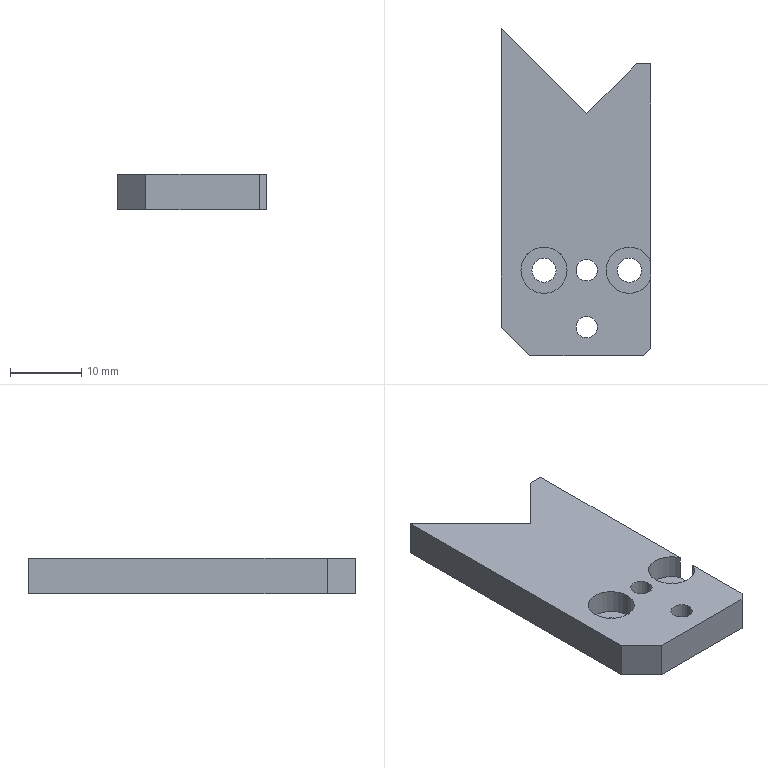Part | STEP file | 11-FG-E02611 | 1 solid | 23 faces | box 21 x 46 x 5 mm | volume 3756 mm3 | plane 12 | cylinder 11 | commonest cylinder face diameters 3 x4 3.4 x4 6.5 x3
STEP:
#1=CARTESIAN_POINT('',(1.5,-9.5,0.));
#2=VERTEX_POINT('',#1);
#3=CARTESIAN_POINT('',(-1.5,-9.5,0.));
#4=VERTEX_POINT('',#3);
#5=CARTESIAN_POINT('',(0.,-9.5,0.));
#6=DIRECTION('',(0.,0.,-1.));
#7=DIRECTION('',(-1.,0.,0.));
#8=AXIS2_PLACEMENT_3D('',#5,#6,#7);
#9=CIRCLE('',#8,1.5);
#10=EDGE_CURVE('',#2,#4,#9,.T.);
#11=ORIENTED_EDGE('',*,*,#10,.T.);
#12=CARTESIAN_POINT('',(-1.5,-9.5,5.));
#13=VERTEX_POINT('',#12);
#14=CARTESIAN_POINT('',(-1.5,-9.5,5.));
#15=DIRECTION('',(0.,0.,1.));
#16=VECTOR('',#15,1000.);
#17=LINE('',#14,#16);
#18=EDGE_CURVE('',#4,#13,#17,.T.);
#19=ORIENTED_EDGE('',*,*,#18,.T.);
#20=CARTESIAN_POINT('',(1.5,-9.5,5.));
#21=VERTEX_POINT('',#20);
#22=CARTESIAN_POINT('',(0.,-9.5,5.));
#23=DIRECTION('',(0.,0.,1.));
#24=DIRECTION('',(1.,0.,0.));
#25=AXIS2_PLACEMENT_3D('',#22,#23,#24);
#26=CIRCLE('',#25,1.5);
#27=EDGE_CURVE('',#13,#21,#26,.T.);
#28=ORIENTED_EDGE('',*,*,#27,.T.);
#29=CARTESIAN_POINT('',(1.5,-9.5,5.));
#30=DIRECTION('',(0.,0.,1.));
#31=VECTOR('',#30,1000.);
#32=LINE('',#29,#31);
#33=EDGE_CURVE('',#2,#21,#32,.T.);
#34=ORIENTED_EDGE('',*,*,#33,.F.);
#35=EDGE_LOOP('',(#11,#19,#28,#34));
#36=FACE_OUTER_BOUND('',#35,.T.);
#37=CARTESIAN_POINT('',(0.,-9.5,5.));
#38=DIRECTION('',(0.,0.,1.));
#39=DIRECTION('',(1.,0.,0.));
#40=AXIS2_PLACEMENT_3D('',#37,#38,#39);
#41=CYLINDRICAL_SURFACE('',#40,1.5);
#42=ADVANCED_FACE('',(#36),#41,.F.);
#43=CARTESIAN_POINT('',(1.5,-17.5,0.));
#44=VERTEX_POINT('',#43);
#45=CARTESIAN_POINT('',(-1.5,-17.5,0.));
#46=VERTEX_POINT('',#45);
#47=CARTESIAN_POINT('',(0.,-17.5,0.));
#48=DIRECTION('',(0.,0.,-1.));
#49=DIRECTION('',(-1.,0.,0.));
#50=AXIS2_PLACEMENT_3D('',#47,#48,#49);
#51=CIRCLE('',#50,1.5);
#52=EDGE_CURVE('',#44,#46,#51,.T.);
#53=ORIENTED_EDGE('',*,*,#52,.T.);
#54=CARTESIAN_POINT('',(-1.5,-17.5,5.));
#55=VERTEX_POINT('',#54);
#56=CARTESIAN_POINT('',(-1.5,-17.5,5.));
#57=DIRECTION('',(0.,0.,1.));
#58=VECTOR('',#57,1000.);
#59=LINE('',#56,#58);
#60=EDGE_CURVE('',#46,#55,#59,.T.);
#61=ORIENTED_EDGE('',*,*,#60,.T.);
#62=CARTESIAN_POINT('',(1.5,-17.5,5.));
#63=VERTEX_POINT('',#62);
#64=CARTESIAN_POINT('',(0.,-17.5,5.));
#65=DIRECTION('',(0.,0.,1.));
#66=DIRECTION('',(1.,0.,0.));
#67=AXIS2_PLACEMENT_3D('',#64,#65,#66);
#68=CIRCLE('',#67,1.5);
#69=EDGE_CURVE('',#55,#63,#68,.T.);
#70=ORIENTED_EDGE('',*,*,#69,.T.);
#71=CARTESIAN_POINT('',(1.5,-17.5,5.));
#72=DIRECTION('',(0.,0.,1.));
#73=VECTOR('',#72,1000.);
#74=LINE('',#71,#73);
#75=EDGE_CURVE('',#44,#63,#74,.T.);
#76=ORIENTED_EDGE('',*,*,#75,.F.);
#77=EDGE_LOOP('',(#53,#61,#70,#76));
#78=FACE_OUTER_BOUND('',#77,.T.);
#79=CARTESIAN_POINT('',(0.,-17.5,5.));
#80=DIRECTION('',(0.,0.,1.));
#81=DIRECTION('',(1.,0.,0.));
#82=AXIS2_PLACEMENT_3D('',#79,#80,#81);
#83=CYLINDRICAL_SURFACE('',#82,1.5);
#84=ADVANCED_FACE('',(#78),#83,.F.);
#85=CARTESIAN_POINT('',(4.3,-9.5,0.));
#86=VERTEX_POINT('',#85);
#87=CARTESIAN_POINT('',(7.7,-9.5,0.));
#88=VERTEX_POINT('',#87);
#89=CARTESIAN_POINT('',(6.,-9.5,0.));
#90=DIRECTION('',(0.,0.,1.));
#91=DIRECTION('',(1.,0.,0.));
#92=AXIS2_PLACEMENT_3D('',#89,#90,#91);
#93=CIRCLE('',#92,1.7);
#94=EDGE_CURVE('',#86,#88,#93,.T.);
#95=ORIENTED_EDGE('',*,*,#94,.F.);
#96=CARTESIAN_POINT('',(4.3,-9.5,1.6));
#97=VERTEX_POINT('',#96);
#98=CARTESIAN_POINT('',(4.3,-9.5,5.));
#99=DIRECTION('',(0.,0.,1.));
#100=VECTOR('',#99,1000.);
#101=LINE('',#98,#100);
#102=EDGE_CURVE('',#86,#97,#101,.T.);
#103=ORIENTED_EDGE('',*,*,#102,.T.);
#104=CARTESIAN_POINT('',(7.7,-9.5,1.6));
#105=VERTEX_POINT('',#104);
#106=CARTESIAN_POINT('',(6.,-9.5,1.6));
#107=DIRECTION('',(0.,0.,1.));
#108=DIRECTION('',(1.,0.,0.));
#109=AXIS2_PLACEMENT_3D('',#106,#107,#108);
#110=CIRCLE('',#109,1.7);
#111=EDGE_CURVE('',#97,#105,#110,.T.);
#112=ORIENTED_EDGE('',*,*,#111,.T.);
#113=CARTESIAN_POINT('',(7.7,-9.5,5.));
#114=DIRECTION('',(0.,0.,1.));
#115=VECTOR('',#114,1000.);
#116=LINE('',#113,#115);
#117=EDGE_CURVE('',#88,#105,#116,.T.);
#118=ORIENTED_EDGE('',*,*,#117,.F.);
#119=EDGE_LOOP('',(#95,#103,#112,#118));
#120=FACE_OUTER_BOUND('',#119,.T.);
#121=CARTESIAN_POINT('',(6.,-9.5,5.));
#122=DIRECTION('',(0.,0.,1.));
#123=DIRECTION('',(1.,0.,0.));
#124=AXIS2_PLACEMENT_3D('',#121,#122,#123);
#125=CYLINDRICAL_SURFACE('',#124,1.7);
#126=ADVANCED_FACE('',(#120),#125,.F.);
#127=CARTESIAN_POINT('',(-7.7,-9.5,0.));
#128=VERTEX_POINT('',#127);
#129=CARTESIAN_POINT('',(-4.3,-9.5,0.));
#130=VERTEX_POINT('',#129);
#131=CARTESIAN_POINT('',(-6.,-9.5,0.));
#132=DIRECTION('',(0.,0.,1.));
#133=DIRECTION('',(1.,0.,0.));
#134=AXIS2_PLACEMENT_3D('',#131,#132,#133);
#135=CIRCLE('',#134,1.7);
#136=EDGE_CURVE('',#128,#130,#135,.T.);
#137=ORIENTED_EDGE('',*,*,#136,.F.);
#138=CARTESIAN_POINT('',(-7.7,-9.5,1.6));
#139=VERTEX_POINT('',#138);
#140=CARTESIAN_POINT('',(-7.7,-9.5,5.));
#141=DIRECTION('',(0.,0.,1.));
#142=VECTOR('',#141,1000.);
#143=LINE('',#140,#142);
#144=EDGE_CURVE('',#128,#139,#143,.T.);
#145=ORIENTED_EDGE('',*,*,#144,.T.);
#146=CARTESIAN_POINT('',(-4.3,-9.5,1.6));
#147=VERTEX_POINT('',#146);
#148=CARTESIAN_POINT('',(-6.,-9.5,1.6));
#149=DIRECTION('',(0.,0.,1.));
#150=DIRECTION('',(1.,0.,0.));
#151=AXIS2_PLACEMENT_3D('',#148,#149,#150);
#152=CIRCLE('',#151,1.7);
#153=EDGE_CURVE('',#139,#147,#152,.T.);
#154=ORIENTED_EDGE('',*,*,#153,.T.);
#155=CARTESIAN_POINT('',(-4.3,-9.5,5.));
#156=DIRECTION('',(0.,0.,1.));
#157=VECTOR('',#156,1000.);
#158=LINE('',#155,#157);
#159=EDGE_CURVE('',#130,#147,#158,.T.);
#160=ORIENTED_EDGE('',*,*,#159,.F.);
#161=EDGE_LOOP('',(#137,#145,#154,#160));
#162=FACE_OUTER_BOUND('',#161,.T.);
#163=CARTESIAN_POINT('',(-6.,-9.5,5.));
#164=DIRECTION('',(0.,0.,1.));
#165=DIRECTION('',(1.,0.,0.));
#166=AXIS2_PLACEMENT_3D('',#163,#164,#165);
#167=CYLINDRICAL_SURFACE('',#166,1.7);
#168=ADVANCED_FACE('',(#162),#167,.F.);
#169=CARTESIAN_POINT('',(-9.25,-9.5,1.6));
#170=VERTEX_POINT('',#169);
#171=CARTESIAN_POINT('',(-2.75,-9.5,1.6));
#172=VERTEX_POINT('',#171);
#173=CARTESIAN_POINT('',(-6.,-9.5,1.6));
#174=DIRECTION('',(0.,0.,1.));
#175=DIRECTION('',(1.,0.,0.));
#176=AXIS2_PLACEMENT_3D('',#173,#174,#175);
#177=CIRCLE('',#176,3.25);
#178=EDGE_CURVE('',#170,#172,#177,.T.);
#179=ORIENTED_EDGE('',*,*,#178,.F.);
#180=CARTESIAN_POINT('',(-9.25,-9.5,5.));
#181=VERTEX_POINT('',#180);
#182=CARTESIAN_POINT('',(-9.25,-9.5,5.));
#183=DIRECTION('',(0.,0.,1.));
#184=VECTOR('',#183,1000.);
#185=LINE('',#182,#184);
#186=EDGE_CURVE('',#170,#181,#185,.T.);
#187=ORIENTED_EDGE('',*,*,#186,.T.);
#188=CARTESIAN_POINT('',(-2.75,-9.5,5.));
#189=VERTEX_POINT('',#188);
#190=CARTESIAN_POINT('',(-6.,-9.5,5.));
#191=DIRECTION('',(0.,0.,1.));
#192=DIRECTION('',(1.,0.,0.));
#193=AXIS2_PLACEMENT_3D('',#190,#191,#192);
#194=CIRCLE('',#193,3.25);
#195=EDGE_CURVE('',#181,#189,#194,.T.);
#196=ORIENTED_EDGE('',*,*,#195,.T.);
#197=CARTESIAN_POINT('',(-2.75,-9.5,5.));
#198=DIRECTION('',(0.,0.,1.));
#199=VECTOR('',#198,1000.);
#200=LINE('',#197,#199);
#201=EDGE_CURVE('',#172,#189,#200,.T.);
#202=ORIENTED_EDGE('',*,*,#201,.F.);
#203=EDGE_LOOP('',(#179,#187,#196,#202));
#204=FACE_OUTER_BOUND('',#203,.T.);
#205=CARTESIAN_POINT('',(-6.,-9.5,5.));
#206=DIRECTION('',(0.,0.,1.));
#207=DIRECTION('',(1.,0.,0.));
#208=AXIS2_PLACEMENT_3D('',#205,#206,#207);
#209=CYLINDRICAL_SURFACE('',#208,3.25);
#210=ADVANCED_FACE('',(#204),#209,.F.);
#211=CARTESIAN_POINT('',(-6.,-9.5,5.));
#212=DIRECTION('',(0.,0.,1.));
#213=DIRECTION('',(1.,0.,0.));
#214=AXIS2_PLACEMENT_3D('',#211,#212,#213);
#215=CIRCLE('',#214,3.25);
#216=EDGE_CURVE('',#189,#181,#215,.T.);
#217=ORIENTED_EDGE('',*,*,#216,.F.);
#218=ORIENTED_EDGE('',*,*,#195,.F.);
#219=EDGE_LOOP('',(#217,#218));
#220=FACE_BOUND('',#219,.T.);
#221=CARTESIAN_POINT('',(0.,-9.5,5.));
#222=DIRECTION('',(0.,0.,1.));
#223=DIRECTION('',(1.,0.,0.));
#224=AXIS2_PLACEMENT_3D('',#221,#222,#223);
#225=CIRCLE('',#224,1.5);
#226=EDGE_CURVE('',#21,#13,#225,.T.);
#227=ORIENTED_EDGE('',*,*,#226,.F.);
#228=ORIENTED_EDGE('',*,*,#27,.F.);
#229=EDGE_LOOP('',(#227,#228));
#230=FACE_BOUND('',#229,.T.);
#231=CARTESIAN_POINT('',(0.,-17.5,5.));
#232=DIRECTION('',(0.,0.,1.));
#233=DIRECTION('',(1.,0.,0.));
#234=AXIS2_PLACEMENT_3D('',#231,#232,#233);
#235=CIRCLE('',#234,1.5);
#236=EDGE_CURVE('',#63,#55,#235,.T.);
#237=ORIENTED_EDGE('',*,*,#236,.F.);
#238=ORIENTED_EDGE('',*,*,#69,.F.);
#239=EDGE_LOOP('',(#237,#238));
#240=FACE_BOUND('',#239,.T.);
#241=CARTESIAN_POINT('',(-8.,-21.5,5.));
#242=VERTEX_POINT('',#241);
#243=CARTESIAN_POINT('',(8.,-21.5,5.));
#244=VERTEX_POINT('',#243);
#245=CARTESIAN_POINT('',(-9.,-21.5,5.));
#246=DIRECTION('',(1.,0.,0.));
#247=VECTOR('',#246,1000.);
#248=LINE('',#245,#247);
#249=EDGE_CURVE('',#242,#244,#248,.T.);
#250=ORIENTED_EDGE('',*,*,#249,.T.);
#251=CARTESIAN_POINT('',(9.,-20.5,5.));
#252=VERTEX_POINT('',#251);
#253=CARTESIAN_POINT('',(9.,-20.5,5.));
#254=DIRECTION('',(0.7071,0.7071,0.));
#255=VECTOR('',#254,1000.);
#256=LINE('',#253,#255);
#257=EDGE_CURVE('',#244,#252,#256,.T.);
#258=ORIENTED_EDGE('',*,*,#257,.T.);
#259=CARTESIAN_POINT('',(9.,-10.75,5.));
#260=VERTEX_POINT('',#259);
#261=CARTESIAN_POINT('',(9.,-21.5,5.));
#262=DIRECTION('',(0.,1.,0.));
#263=VECTOR('',#262,1000.);
#264=LINE('',#261,#263);
#265=EDGE_CURVE('',#252,#260,#264,.T.);
#266=ORIENTED_EDGE('',*,*,#265,.T.);
#267=CARTESIAN_POINT('',(9.,-8.25,5.));
#268=VERTEX_POINT('',#267);
#269=CARTESIAN_POINT('',(6.,-9.5,5.));
#270=DIRECTION('',(0.,0.,1.));
#271=DIRECTION('',(1.,0.,0.));
#272=AXIS2_PLACEMENT_3D('',#269,#270,#271);
#273=CIRCLE('',#272,3.25);
#274=EDGE_CURVE('',#268,#260,#273,.T.);
#275=ORIENTED_EDGE('',*,*,#274,.F.);
#276=CARTESIAN_POINT('',(9.,19.5,5.));
#277=VERTEX_POINT('',#276);
#278=CARTESIAN_POINT('',(9.,-21.5,5.));
#279=DIRECTION('',(0.,1.,0.));
#280=VECTOR('',#279,1000.);
#281=LINE('',#278,#280);
#282=EDGE_CURVE('',#268,#277,#281,.T.);
#283=ORIENTED_EDGE('',*,*,#282,.T.);
#284=CARTESIAN_POINT('',(7.,19.5,5.));
#285=VERTEX_POINT('',#284);
#286=CARTESIAN_POINT('',(0.,19.5,5.));
#287=DIRECTION('',(1.,0.,0.));
#288=VECTOR('',#287,1000.);
#289=LINE('',#286,#288);
#290=EDGE_CURVE('',#285,#277,#289,.T.);
#291=ORIENTED_EDGE('',*,*,#290,.F.);
#292=CARTESIAN_POINT('',(0.,12.5,5.));
#293=VERTEX_POINT('',#292);
#294=CARTESIAN_POINT('',(0.,12.5,5.));
#295=DIRECTION('',(0.7071,0.7071,0.));
#296=VECTOR('',#295,1000.);
#297=LINE('',#294,#296);
#298=EDGE_CURVE('',#293,#285,#297,.T.);
#299=ORIENTED_EDGE('',*,*,#298,.F.);
#300=CARTESIAN_POINT('',(-12.,24.5,5.));
#301=VERTEX_POINT('',#300);
#302=CARTESIAN_POINT('',(-9.,21.5,5.));
#303=DIRECTION('',(0.7071,-0.7071,0.));
#304=VECTOR('',#303,1000.);
#305=LINE('',#302,#304);
#306=EDGE_CURVE('',#301,#293,#305,.T.);
#307=ORIENTED_EDGE('',*,*,#306,.F.);
#308=CARTESIAN_POINT('',(-12.,-17.5,5.));
#309=VERTEX_POINT('',#308);
#310=CARTESIAN_POINT('',(-12.,0.,5.));
#311=DIRECTION('',(0.,-1.,0.));
#312=VECTOR('',#311,1000.);
#313=LINE('',#310,#312);
#314=EDGE_CURVE('',#301,#309,#313,.T.);
#315=ORIENTED_EDGE('',*,*,#314,.T.);
#316=CARTESIAN_POINT('',(-8.,-21.5,5.));
#317=DIRECTION('',(0.7071,-0.7071,0.));
#318=VECTOR('',#317,1000.);
#319=LINE('',#316,#318);
#320=EDGE_CURVE('',#309,#242,#319,.T.);
#321=ORIENTED_EDGE('',*,*,#320,.T.);
#322=EDGE_LOOP('',(#250,#258,#266,#275,#283,#291,#299,#307,#315,#321));
#323=FACE_OUTER_BOUND('',#322,.T.);
#324=CARTESIAN_POINT('',(0.,0.,5.));
#325=DIRECTION('',(0.,0.,-1.));
#326=DIRECTION('',(-1.,0.,0.));
#327=AXIS2_PLACEMENT_3D('',#324,#325,#326);
#328=PLANE('',#327);
#329=ADVANCED_FACE('',(#220,#230,#240,#323),#328,.F.);
#330=ORIENTED_EDGE('',*,*,#265,.F.);
#331=CARTESIAN_POINT('',(9.,-20.5,0.));
#332=VERTEX_POINT('',#331);
#333=CARTESIAN_POINT('',(9.,-20.5,5.));
#334=DIRECTION('',(0.,0.,-1.));
#335=VECTOR('',#334,1000.);
#336=LINE('',#333,#335);
#337=EDGE_CURVE('',#252,#332,#336,.T.);
#338=ORIENTED_EDGE('',*,*,#337,.T.);
#339=CARTESIAN_POINT('',(9.,19.5,0.));
#340=VERTEX_POINT('',#339);
#341=CARTESIAN_POINT('',(9.,-21.5,0.));
#342=DIRECTION('',(0.,1.,0.));
#343=VECTOR('',#342,1000.);
#344=LINE('',#341,#343);
#345=EDGE_CURVE('',#332,#340,#344,.T.);
#346=ORIENTED_EDGE('',*,*,#345,.T.);
#347=CARTESIAN_POINT('',(9.,19.5,-5.));
#348=DIRECTION('',(0.,0.,1.));
#349=VECTOR('',#348,1000.);
#350=LINE('',#347,#349);
#351=EDGE_CURVE('',#340,#277,#350,.T.);
#352=ORIENTED_EDGE('',*,*,#351,.T.);
#353=ORIENTED_EDGE('',*,*,#282,.F.);
#354=CARTESIAN_POINT('',(9.,-8.25,1.6));
#355=VERTEX_POINT('',#354);
#356=CARTESIAN_POINT('',(9.,-8.25,5.));
#357=DIRECTION('',(0.,0.,-1.));
#358=VECTOR('',#357,1000.);
#359=LINE('',#356,#358);
#360=EDGE_CURVE('',#268,#355,#359,.T.);
#361=ORIENTED_EDGE('',*,*,#360,.T.);
#362=CARTESIAN_POINT('',(9.,-10.75,1.6));
#363=VERTEX_POINT('',#362);
#364=CARTESIAN_POINT('',(9.,-21.5,1.6));
#365=DIRECTION('',(0.,-1.,0.));
#366=VECTOR('',#365,1000.);
#367=LINE('',#364,#366);
#368=EDGE_CURVE('',#355,#363,#367,.T.);
#369=ORIENTED_EDGE('',*,*,#368,.T.);
#370=CARTESIAN_POINT('',(9.,-10.75,5.));
#371=DIRECTION('',(0.,0.,1.));
#372=VECTOR('',#371,1000.);
#373=LINE('',#370,#372);
#374=EDGE_CURVE('',#363,#260,#373,.T.);
#375=ORIENTED_EDGE('',*,*,#374,.T.);
#376=EDGE_LOOP('',(#330,#338,#346,#352,#353,#361,#369,#375));
#377=FACE_OUTER_BOUND('',#376,.T.);
#378=CARTESIAN_POINT('',(9.,-21.5,5.));
#379=DIRECTION('',(-1.,0.,0.));
#380=DIRECTION('',(0.,0.,1.));
#381=AXIS2_PLACEMENT_3D('',#378,#379,#380);
#382=PLANE('',#381);
#383=ADVANCED_FACE('',(#377),#382,.F.);
#384=CARTESIAN_POINT('',(-12.,24.5,0.));
#385=VERTEX_POINT('',#384);
#386=CARTESIAN_POINT('',(-12.,-17.5,0.));
#387=VERTEX_POINT('',#386);
#388=CARTESIAN_POINT('',(-12.,0.,0.));
#389=DIRECTION('',(0.,-1.,0.));
#390=VECTOR('',#389,1000.);
#391=LINE('',#388,#390);
#392=EDGE_CURVE('',#385,#387,#391,.T.);
#393=ORIENTED_EDGE('',*,*,#392,.T.);
#394=CARTESIAN_POINT('',(-12.,-17.5,5.));
#395=DIRECTION('',(0.,0.,1.));
#396=VECTOR('',#395,1000.);
#397=LINE('',#394,#396);
#398=EDGE_CURVE('',#387,#309,#397,.T.);
#399=ORIENTED_EDGE('',*,*,#398,.T.);
#400=ORIENTED_EDGE('',*,*,#314,.F.);
#401=CARTESIAN_POINT('',(-12.,24.5,5.));
#402=DIRECTION('',(0.,0.,-1.));
#403=VECTOR('',#402,1000.);
#404=LINE('',#401,#403);
#405=EDGE_CURVE('',#301,#385,#404,.T.);
#406=ORIENTED_EDGE('',*,*,#405,.T.);
#407=EDGE_LOOP('',(#393,#399,#400,#406));
#408=FACE_OUTER_BOUND('',#407,.T.);
#409=CARTESIAN_POINT('',(-12.,-21.5,5.));
#410=DIRECTION('',(1.,0.,0.));
#411=DIRECTION('',(0.,0.,-1.));
#412=AXIS2_PLACEMENT_3D('',#409,#410,#411);
#413=PLANE('',#412);
#414=ADVANCED_FACE('',(#408),#413,.F.);
#415=CARTESIAN_POINT('',(-8.,-21.5,0.));
#416=VERTEX_POINT('',#415);
#417=CARTESIAN_POINT('',(8.,-21.5,0.));
#418=VERTEX_POINT('',#417);
#419=CARTESIAN_POINT('',(-9.,-21.5,0.));
#420=DIRECTION('',(1.,0.,0.));
#421=VECTOR('',#420,1000.);
#422=LINE('',#419,#421);
#423=EDGE_CURVE('',#416,#418,#422,.T.);
#424=ORIENTED_EDGE('',*,*,#423,.T.);
#425=CARTESIAN_POINT('',(8.,-21.5,5.));
#426=DIRECTION('',(0.,0.,1.));
#427=VECTOR('',#426,1000.);
#428=LINE('',#425,#427);
#429=EDGE_CURVE('',#418,#244,#428,.T.);
#430=ORIENTED_EDGE('',*,*,#429,.T.);
#431=ORIENTED_EDGE('',*,*,#249,.F.);
#432=CARTESIAN_POINT('',(-8.,-21.5,5.));
#433=DIRECTION('',(0.,0.,-1.));
#434=VECTOR('',#433,1000.);
#435=LINE('',#432,#434);
#436=EDGE_CURVE('',#242,#416,#435,.T.);
#437=ORIENTED_EDGE('',*,*,#436,.T.);
#438=EDGE_LOOP('',(#424,#430,#431,#437));
#439=FACE_OUTER_BOUND('',#438,.T.);
#440=CARTESIAN_POINT('',(-9.,-21.5,5.));
#441=DIRECTION('',(0.,1.,0.));
#442=DIRECTION('',(0.,0.,1.));
#443=AXIS2_PLACEMENT_3D('',#440,#441,#442);
#444=PLANE('',#443);
#445=ADVANCED_FACE('',(#439),#444,.F.);
#446=ORIENTED_EDGE('',*,*,#10,.F.);
#447=CARTESIAN_POINT('',(0.,-9.5,0.));
#448=DIRECTION('',(0.,0.,-1.));
#449=DIRECTION('',(-1.,0.,0.));
#450=AXIS2_PLACEMENT_3D('',#447,#448,#449);
#451=CIRCLE('',#450,1.5);
#452=EDGE_CURVE('',#4,#2,#451,.T.);
#453=ORIENTED_EDGE('',*,*,#452,.F.);
#454=EDGE_LOOP('',(#446,#453));
#455=FACE_BOUND('',#454,.T.);
#456=ORIENTED_EDGE('',*,*,#52,.F.);
#457=CARTESIAN_POINT('',(0.,-17.5,0.));
#458=DIRECTION('',(0.,0.,-1.));
#459=DIRECTION('',(-1.,0.,0.));
#460=AXIS2_PLACEMENT_3D('',#457,#458,#459);
#461=CIRCLE('',#460,1.5);
#462=EDGE_CURVE('',#46,#44,#461,.T.);
#463=ORIENTED_EDGE('',*,*,#462,.F.);
#464=EDGE_LOOP('',(#456,#463));
#465=FACE_BOUND('',#464,.T.);
#466=ORIENTED_EDGE('',*,*,#345,.F.);
#467=CARTESIAN_POINT('',(14.75,-14.75,0.));
#468=DIRECTION('',(-0.7071,-0.7071,0.));
#469=VECTOR('',#468,1000.);
#470=LINE('',#467,#469);
#471=EDGE_CURVE('',#332,#418,#470,.T.);
#472=ORIENTED_EDGE('',*,*,#471,.T.);
#473=ORIENTED_EDGE('',*,*,#423,.F.);
#474=CARTESIAN_POINT('',(-14.75,-14.75,0.));
#475=DIRECTION('',(-0.7071,0.7071,0.));
#476=VECTOR('',#475,1000.);
#477=LINE('',#474,#476);
#478=EDGE_CURVE('',#416,#387,#477,.T.);
#479=ORIENTED_EDGE('',*,*,#478,.T.);
#480=ORIENTED_EDGE('',*,*,#392,.F.);
#481=CARTESIAN_POINT('',(0.,12.5,0.));
#482=VERTEX_POINT('',#481);
#483=CARTESIAN_POINT('',(-9.,21.5,0.));
#484=DIRECTION('',(0.7071,-0.7071,0.));
#485=VECTOR('',#484,1000.);
#486=LINE('',#483,#485);
#487=EDGE_CURVE('',#385,#482,#486,.T.);
#488=ORIENTED_EDGE('',*,*,#487,.T.);
#489=CARTESIAN_POINT('',(7.,19.5,0.));
#490=VERTEX_POINT('',#489);
#491=CARTESIAN_POINT('',(0.,12.5,0.));
#492=DIRECTION('',(0.7071,0.7071,0.));
#493=VECTOR('',#492,1000.);
#494=LINE('',#491,#493);
#495=EDGE_CURVE('',#482,#490,#494,.T.);
#496=ORIENTED_EDGE('',*,*,#495,.T.);
#497=CARTESIAN_POINT('',(0.,19.5,0.));
#498=DIRECTION('',(-1.,0.,0.));
#499=VECTOR('',#498,1000.);
#500=LINE('',#497,#499);
#501=EDGE_CURVE('',#340,#490,#500,.T.);
#502=ORIENTED_EDGE('',*,*,#501,.F.);
#503=EDGE_LOOP('',(#466,#472,#473,#479,#480,#488,#496,#502));
#504=FACE_OUTER_BOUND('',#503,.T.);
#505=CARTESIAN_POINT('',(6.,-9.5,0.));
#506=DIRECTION('',(0.,0.,1.));
#507=DIRECTION('',(1.,0.,0.));
#508=AXIS2_PLACEMENT_3D('',#505,#506,#507);
#509=CIRCLE('',#508,1.7);
#510=EDGE_CURVE('',#88,#86,#509,.T.);
#511=ORIENTED_EDGE('',*,*,#510,.T.);
#512=ORIENTED_EDGE('',*,*,#94,.T.);
#513=EDGE_LOOP('',(#511,#512));
#514=FACE_BOUND('',#513,.T.);
#515=CARTESIAN_POINT('',(-6.,-9.5,0.));
#516=DIRECTION('',(0.,0.,1.));
#517=DIRECTION('',(1.,0.,0.));
#518=AXIS2_PLACEMENT_3D('',#515,#516,#517);
#519=CIRCLE('',#518,1.7);
#520=EDGE_CURVE('',#130,#128,#519,.T.);
#521=ORIENTED_EDGE('',*,*,#520,.T.);
#522=ORIENTED_EDGE('',*,*,#136,.T.);
#523=EDGE_LOOP('',(#521,#522));
#524=FACE_BOUND('',#523,.T.);
#525=CARTESIAN_POINT('',(0.,0.,0.));
#526=DIRECTION('',(0.,0.,-1.));
#527=DIRECTION('',(-1.,0.,0.));
#528=AXIS2_PLACEMENT_3D('',#525,#526,#527);
#529=PLANE('',#528);
#530=ADVANCED_FACE('',(#455,#465,#504,#514,#524),#529,.T.);
#531=ORIENTED_EDGE('',*,*,#298,.T.);
#532=CARTESIAN_POINT('',(7.,19.5,0.));
#533=DIRECTION('',(0.,0.,-1.));
#534=VECTOR('',#533,1000.);
#535=LINE('',#532,#534);
#536=EDGE_CURVE('',#285,#490,#535,.T.);
#537=ORIENTED_EDGE('',*,*,#536,.T.);
#538=ORIENTED_EDGE('',*,*,#495,.F.);
#539=CARTESIAN_POINT('',(0.,12.5,0.));
#540=DIRECTION('',(0.,0.,1.));
#541=VECTOR('',#540,1000.);
#542=LINE('',#539,#541);
#543=EDGE_CURVE('',#482,#293,#542,.T.);
#544=ORIENTED_EDGE('',*,*,#543,.T.);
#545=EDGE_LOOP('',(#531,#537,#538,#544));
#546=FACE_OUTER_BOUND('',#545,.T.);
#547=CARTESIAN_POINT('',(0.,12.5,0.));
#548=DIRECTION('',(0.7071,-0.7071,0.));
#549=DIRECTION('',(0.7071,0.7071,0.));
#550=AXIS2_PLACEMENT_3D('',#547,#548,#549);
#551=PLANE('',#550);
#552=ADVANCED_FACE('',(#546),#551,.F.);
#553=ORIENTED_EDGE('',*,*,#306,.T.);
#554=ORIENTED_EDGE('',*,*,#543,.F.);
#555=ORIENTED_EDGE('',*,*,#487,.F.);
#556=ORIENTED_EDGE('',*,*,#405,.F.);
#557=EDGE_LOOP('',(#553,#554,#555,#556));
#558=FACE_OUTER_BOUND('',#557,.T.);
#559=CARTESIAN_POINT('',(-9.,21.5,0.));
#560=DIRECTION('',(-0.7071,-0.7071,0.));
#561=DIRECTION('',(0.7071,-0.7071,0.));
#562=AXIS2_PLACEMENT_3D('',#559,#560,#561);
#563=PLANE('',#562);
#564=ADVANCED_FACE('',(#558),#563,.F.);
#565=CARTESIAN_POINT('',(-6.,-9.5,1.6));
#566=DIRECTION('',(0.,0.,1.));
#567=DIRECTION('',(1.,0.,0.));
#568=AXIS2_PLACEMENT_3D('',#565,#566,#567);
#569=CIRCLE('',#568,1.7);
#570=EDGE_CURVE('',#147,#139,#569,.T.);
#571=ORIENTED_EDGE('',*,*,#570,.F.);
#572=ORIENTED_EDGE('',*,*,#153,.F.);
#573=EDGE_LOOP('',(#571,#572));
#574=FACE_BOUND('',#573,.T.);
#575=CARTESIAN_POINT('',(-6.,-9.5,1.6));
#576=DIRECTION('',(0.,0.,1.));
#577=DIRECTION('',(1.,0.,0.));
#578=AXIS2_PLACEMENT_3D('',#575,#576,#577);
#579=CIRCLE('',#578,3.25);
#580=EDGE_CURVE('',#172,#170,#579,.T.);
#581=ORIENTED_EDGE('',*,*,#580,.T.);
#582=ORIENTED_EDGE('',*,*,#178,.T.);
#583=EDGE_LOOP('',(#581,#582));
#584=FACE_OUTER_BOUND('',#583,.T.);
#585=CARTESIAN_POINT('',(-4.3,-9.5,1.6));
#586=DIRECTION('',(0.,0.,-1.));
#587=DIRECTION('',(-1.,0.,0.));
#588=AXIS2_PLACEMENT_3D('',#585,#586,#587);
#589=PLANE('',#588);
#590=ADVANCED_FACE('',(#574,#584),#589,.F.);
#591=ORIENTED_EDGE('',*,*,#186,.F.);
#592=ORIENTED_EDGE('',*,*,#580,.F.);
#593=ORIENTED_EDGE('',*,*,#201,.T.);
#594=ORIENTED_EDGE('',*,*,#216,.T.);
#595=EDGE_LOOP('',(#591,#592,#593,#594));
#596=FACE_OUTER_BOUND('',#595,.T.);
#597=CARTESIAN_POINT('',(-6.,-9.5,5.));
#598=DIRECTION('',(0.,0.,1.));
#599=DIRECTION('',(1.,0.,0.));
#600=AXIS2_PLACEMENT_3D('',#597,#598,#599);
#601=CYLINDRICAL_SURFACE('',#600,3.25);
#602=ADVANCED_FACE('',(#596),#601,.F.);
#603=ORIENTED_EDGE('',*,*,#144,.F.);
#604=ORIENTED_EDGE('',*,*,#520,.F.);
#605=ORIENTED_EDGE('',*,*,#159,.T.);
#606=ORIENTED_EDGE('',*,*,#570,.T.);
#607=EDGE_LOOP('',(#603,#604,#605,#606));
#608=FACE_OUTER_BOUND('',#607,.T.);
#609=CARTESIAN_POINT('',(-6.,-9.5,5.));
#610=DIRECTION('',(0.,0.,1.));
#611=DIRECTION('',(1.,0.,0.));
#612=AXIS2_PLACEMENT_3D('',#609,#610,#611);
#613=CYLINDRICAL_SURFACE('',#612,1.7);
#614=ADVANCED_FACE('',(#608),#613,.F.);
#615=CARTESIAN_POINT('',(6.,-9.5,1.6));
#616=DIRECTION('',(0.,0.,1.));
#617=DIRECTION('',(1.,0.,0.));
#618=AXIS2_PLACEMENT_3D('',#615,#616,#617);
#619=CIRCLE('',#618,3.25);
#620=EDGE_CURVE('',#355,#363,#619,.T.);
#621=ORIENTED_EDGE('',*,*,#620,.F.);
#622=ORIENTED_EDGE('',*,*,#360,.F.);
#623=ORIENTED_EDGE('',*,*,#274,.T.);
#624=ORIENTED_EDGE('',*,*,#374,.F.);
#625=EDGE_LOOP('',(#621,#622,#623,#624));
#626=FACE_OUTER_BOUND('',#625,.T.);
#627=CARTESIAN_POINT('',(6.,-9.5,5.));
#628=DIRECTION('',(0.,0.,1.));
#629=DIRECTION('',(1.,0.,0.));
#630=AXIS2_PLACEMENT_3D('',#627,#628,#629);
#631=CYLINDRICAL_SURFACE('',#630,3.25);
#632=ADVANCED_FACE('',(#626),#631,.F.);
#633=CARTESIAN_POINT('',(6.,-9.5,1.6));
#634=DIRECTION('',(0.,0.,1.));
#635=DIRECTION('',(1.,0.,0.));
#636=AXIS2_PLACEMENT_3D('',#633,#634,#635);
#637=CIRCLE('',#636,1.7);
#638=EDGE_CURVE('',#105,#97,#637,.T.);
#639=ORIENTED_EDGE('',*,*,#638,.F.);
#640=ORIENTED_EDGE('',*,*,#111,.F.);
#641=EDGE_LOOP('',(#639,#640));
#642=FACE_BOUND('',#641,.T.);
#643=ORIENTED_EDGE('',*,*,#620,.T.);
#644=ORIENTED_EDGE('',*,*,#368,.F.);
#645=EDGE_LOOP('',(#643,#644));
#646=FACE_OUTER_BOUND('',#645,.T.);
#647=CARTESIAN_POINT('',(7.7,-9.5,1.6));
#648=DIRECTION('',(0.,0.,-1.));
#649=DIRECTION('',(-1.,0.,0.));
#650=AXIS2_PLACEMENT_3D('',#647,#648,#649);
#651=PLANE('',#650);
#652=ADVANCED_FACE('',(#642,#646),#651,.F.);
#653=ORIENTED_EDGE('',*,*,#102,.F.);
#654=ORIENTED_EDGE('',*,*,#510,.F.);
#655=ORIENTED_EDGE('',*,*,#117,.T.);
#656=ORIENTED_EDGE('',*,*,#638,.T.);
#657=EDGE_LOOP('',(#653,#654,#655,#656));
#658=FACE_OUTER_BOUND('',#657,.T.);
#659=CARTESIAN_POINT('',(6.,-9.5,5.));
#660=DIRECTION('',(0.,0.,1.));
#661=DIRECTION('',(1.,0.,0.));
#662=AXIS2_PLACEMENT_3D('',#659,#660,#661);
#663=CYLINDRICAL_SURFACE('',#662,1.7);
#664=ADVANCED_FACE('',(#658),#663,.F.);
#665=ORIENTED_EDGE('',*,*,#501,.T.);
#666=ORIENTED_EDGE('',*,*,#536,.F.);
#667=ORIENTED_EDGE('',*,*,#290,.T.);
#668=ORIENTED_EDGE('',*,*,#351,.F.);
#669=EDGE_LOOP('',(#665,#666,#667,#668));
#670=FACE_OUTER_BOUND('',#669,.T.);
#671=CARTESIAN_POINT('',(0.,19.5,-5.));
#672=DIRECTION('',(0.,-1.,0.));
#673=DIRECTION('',(0.,0.,-1.));
#674=AXIS2_PLACEMENT_3D('',#671,#672,#673);
#675=PLANE('',#674);
#676=ADVANCED_FACE('',(#670),#675,.F.);
#677=ORIENTED_EDGE('',*,*,#60,.F.);
#678=ORIENTED_EDGE('',*,*,#462,.T.);
#679=ORIENTED_EDGE('',*,*,#75,.T.);
#680=ORIENTED_EDGE('',*,*,#236,.T.);
#681=EDGE_LOOP('',(#677,#678,#679,#680));
#682=FACE_OUTER_BOUND('',#681,.T.);
#683=CARTESIAN_POINT('',(0.,-17.5,5.));
#684=DIRECTION('',(0.,0.,1.));
#685=DIRECTION('',(1.,0.,0.));
#686=AXIS2_PLACEMENT_3D('',#683,#684,#685);
#687=CYLINDRICAL_SURFACE('',#686,1.5);
#688=ADVANCED_FACE('',(#682),#687,.F.);
#689=ORIENTED_EDGE('',*,*,#18,.F.);
#690=ORIENTED_EDGE('',*,*,#452,.T.);
#691=ORIENTED_EDGE('',*,*,#33,.T.);
#692=ORIENTED_EDGE('',*,*,#226,.T.);
#693=EDGE_LOOP('',(#689,#690,#691,#692));
#694=FACE_OUTER_BOUND('',#693,.T.);
#695=CARTESIAN_POINT('',(0.,-9.5,5.));
#696=DIRECTION('',(0.,0.,1.));
#697=DIRECTION('',(1.,0.,0.));
#698=AXIS2_PLACEMENT_3D('',#695,#696,#697);
#699=CYLINDRICAL_SURFACE('',#698,1.5);
#700=ADVANCED_FACE('',(#694),#699,.F.);
#701=ORIENTED_EDGE('',*,*,#257,.F.);
#702=ORIENTED_EDGE('',*,*,#429,.F.);
#703=ORIENTED_EDGE('',*,*,#471,.F.);
#704=ORIENTED_EDGE('',*,*,#337,.F.);
#705=EDGE_LOOP('',(#701,#702,#703,#704));
#706=FACE_OUTER_BOUND('',#705,.T.);
#707=CARTESIAN_POINT('',(9.,-20.5,5.));
#708=DIRECTION('',(-0.7071,0.7071,0.));
#709=DIRECTION('',(0.,0.,-1.));
#710=AXIS2_PLACEMENT_3D('',#707,#708,#709);
#711=PLANE('',#710);
#712=ADVANCED_FACE('',(#706),#711,.F.);
#713=ORIENTED_EDGE('',*,*,#320,.F.);
#714=ORIENTED_EDGE('',*,*,#398,.F.);
#715=ORIENTED_EDGE('',*,*,#478,.F.);
#716=ORIENTED_EDGE('',*,*,#436,.F.);
#717=EDGE_LOOP('',(#713,#714,#715,#716));
#718=FACE_OUTER_BOUND('',#717,.T.);
#719=CARTESIAN_POINT('',(-8.,-21.5,5.));
#720=DIRECTION('',(0.7071,0.7071,0.));
#721=DIRECTION('',(0.,0.,-1.));
#722=AXIS2_PLACEMENT_3D('',#719,#720,#721);
#723=PLANE('',#722);
#724=ADVANCED_FACE('',(#718),#723,.F.);
#725=CLOSED_SHELL('',(#42,#84,#126,#168,#210,#329,#383,#414,#445,#530,#552,#564,#590,#602,#614,#632,#652,#664,#676,#688,#700,#712,#724));
#726=MANIFOLD_SOLID_BREP('',#725);
#727=CARTESIAN_POINT('',(0.,0.,0.));
#728=DIRECTION('',(0.,0.,1.));
#729=DIRECTION('',(1.,0.,0.));
#730=AXIS2_PLACEMENT_3D('',#727,#728,#729);
#731=(LENGTH_UNIT()NAMED_UNIT(*)SI_UNIT(.MILLI.,.METRE.));
#732=UNCERTAINTY_MEASURE_WITH_UNIT(LENGTH_MEASURE(0.00001),#731,'','');
#733=(NAMED_UNIT(*)PLANE_ANGLE_UNIT()SI_UNIT($,.RADIAN.));
#734=(NAMED_UNIT(*)SI_UNIT($,.STERADIAN.)SOLID_ANGLE_UNIT());
#735=(GEOMETRIC_REPRESENTATION_CONTEXT(3)GLOBAL_UNCERTAINTY_ASSIGNED_CONTEXT((#732))GLOBAL_UNIT_ASSIGNED_CONTEXT((#731,#733,#734))REPRESENTATION_CONTEXT('',''));
#736=ADVANCED_BREP_SHAPE_REPRESENTATION('',(#726,#730),#735);